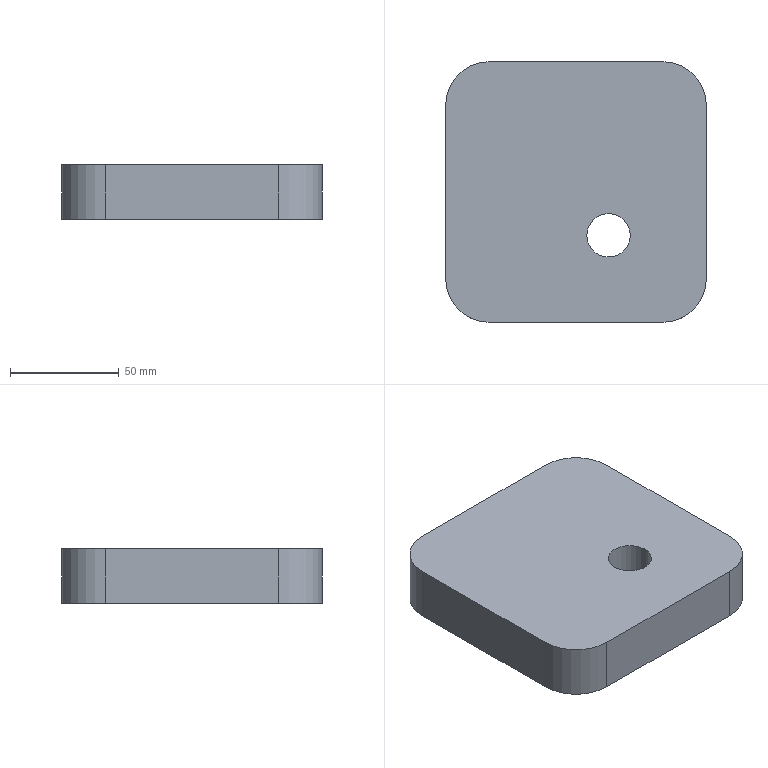Part | SolidWorks | features Extrusion 1, Fillet 1 | 1 solid | 12 faces | box 120 x 120 x 25 mm | volume 343562 mm3 | cylinder 6 | plane 6 | commonest cylinder face diameters 40 x4 20 x2
STEP:
#1=CARTESIAN_POINT('',(65.,40.,25.));
#2=VERTEX_POINT('',#1);
#3=CARTESIAN_POINT('',(85.,40.,25.));
#4=VERTEX_POINT('',#3);
#5=CARTESIAN_POINT('',(75.,40.,25.));
#6=DIRECTION('',(0.,0.,1.));
#7=DIRECTION('',(1.,0.,0.));
#8=AXIS2_PLACEMENT_3D('',#5,#6,#7);
#9=CIRCLE('',#8,10.);
#10=EDGE_CURVE('',#2,#4,#9,.T.);
#11=ORIENTED_EDGE('',*,*,#10,.T.);
#12=CARTESIAN_POINT('',(85.,40.,0.));
#13=VERTEX_POINT('',#12);
#14=CARTESIAN_POINT('',(85.,40.,25.));
#15=DIRECTION('',(0.,0.,-1.));
#16=VECTOR('',#15,1000.);
#17=LINE('',#14,#16);
#18=EDGE_CURVE('',#4,#13,#17,.T.);
#19=ORIENTED_EDGE('',*,*,#18,.T.);
#20=CARTESIAN_POINT('',(65.,40.,0.));
#21=VERTEX_POINT('',#20);
#22=CARTESIAN_POINT('',(75.,40.,0.));
#23=DIRECTION('',(0.,0.,1.));
#24=DIRECTION('',(1.,0.,0.));
#25=AXIS2_PLACEMENT_3D('',#22,#23,#24);
#26=CIRCLE('',#25,10.);
#27=EDGE_CURVE('',#21,#13,#26,.T.);
#28=ORIENTED_EDGE('',*,*,#27,.F.);
#29=CARTESIAN_POINT('',(65.,40.,25.));
#30=DIRECTION('',(0.,0.,-1.));
#31=VECTOR('',#30,1000.);
#32=LINE('',#29,#31);
#33=EDGE_CURVE('',#2,#21,#32,.T.);
#34=ORIENTED_EDGE('',*,*,#33,.F.);
#35=EDGE_LOOP('',(#11,#19,#28,#34));
#36=FACE_OUTER_BOUND('',#35,.T.);
#37=CARTESIAN_POINT('',(75.,40.,25.));
#38=DIRECTION('',(0.,0.,-1.));
#39=DIRECTION('',(-1.,0.,0.));
#40=AXIS2_PLACEMENT_3D('',#37,#38,#39);
#41=CYLINDRICAL_SURFACE('',#40,10.);
#42=ADVANCED_FACE('',(#36),#41,.F.);
#43=CARTESIAN_POINT('',(0.,100.,25.));
#44=VERTEX_POINT('',#43);
#45=CARTESIAN_POINT('',(0.,20.,25.));
#46=VERTEX_POINT('',#45);
#47=CARTESIAN_POINT('',(0.,0.,25.));
#48=DIRECTION('',(0.,-1.,0.));
#49=VECTOR('',#48,1000.);
#50=LINE('',#47,#49);
#51=EDGE_CURVE('',#44,#46,#50,.T.);
#52=ORIENTED_EDGE('',*,*,#51,.T.);
#53=CARTESIAN_POINT('',(20.,0.,25.));
#54=VERTEX_POINT('',#53);
#55=CARTESIAN_POINT('',(20.,20.,25.));
#56=DIRECTION('',(0.,0.,1.));
#57=DIRECTION('',(-1.,0.,0.));
#58=AXIS2_PLACEMENT_3D('',#55,#56,#57);
#59=CIRCLE('',#58,20.);
#60=EDGE_CURVE('',#46,#54,#59,.T.);
#61=ORIENTED_EDGE('',*,*,#60,.T.);
#62=CARTESIAN_POINT('',(100.,0.,25.));
#63=VERTEX_POINT('',#62);
#64=CARTESIAN_POINT('',(0.,0.,25.));
#65=DIRECTION('',(1.,0.,0.));
#66=VECTOR('',#65,1000.);
#67=LINE('',#64,#66);
#68=EDGE_CURVE('',#54,#63,#67,.T.);
#69=ORIENTED_EDGE('',*,*,#68,.T.);
#70=CARTESIAN_POINT('',(120.,20.,25.));
#71=VERTEX_POINT('',#70);
#72=CARTESIAN_POINT('',(100.,20.,25.));
#73=DIRECTION('',(0.,0.,1.));
#74=DIRECTION('',(-1.,0.,0.));
#75=AXIS2_PLACEMENT_3D('',#72,#73,#74);
#76=CIRCLE('',#75,20.);
#77=EDGE_CURVE('',#63,#71,#76,.T.);
#78=ORIENTED_EDGE('',*,*,#77,.T.);
#79=CARTESIAN_POINT('',(120.,100.,25.));
#80=VERTEX_POINT('',#79);
#81=CARTESIAN_POINT('',(120.,0.,25.));
#82=DIRECTION('',(0.,1.,0.));
#83=VECTOR('',#82,1000.);
#84=LINE('',#81,#83);
#85=EDGE_CURVE('',#71,#80,#84,.T.);
#86=ORIENTED_EDGE('',*,*,#85,.T.);
#87=CARTESIAN_POINT('',(100.,120.,25.));
#88=VERTEX_POINT('',#87);
#89=CARTESIAN_POINT('',(100.,100.,25.));
#90=DIRECTION('',(0.,0.,1.));
#91=DIRECTION('',(-1.,0.,0.));
#92=AXIS2_PLACEMENT_3D('',#89,#90,#91);
#93=CIRCLE('',#92,20.);
#94=EDGE_CURVE('',#80,#88,#93,.T.);
#95=ORIENTED_EDGE('',*,*,#94,.T.);
#96=CARTESIAN_POINT('',(20.,120.,25.));
#97=VERTEX_POINT('',#96);
#98=CARTESIAN_POINT('',(0.,120.,25.));
#99=DIRECTION('',(-1.,0.,0.));
#100=VECTOR('',#99,1000.);
#101=LINE('',#98,#100);
#102=EDGE_CURVE('',#88,#97,#101,.T.);
#103=ORIENTED_EDGE('',*,*,#102,.T.);
#104=CARTESIAN_POINT('',(20.,100.,25.));
#105=DIRECTION('',(0.,0.,1.));
#106=DIRECTION('',(-1.,0.,0.));
#107=AXIS2_PLACEMENT_3D('',#104,#105,#106);
#108=CIRCLE('',#107,20.);
#109=EDGE_CURVE('',#97,#44,#108,.T.);
#110=ORIENTED_EDGE('',*,*,#109,.T.);
#111=EDGE_LOOP('',(#52,#61,#69,#78,#86,#95,#103,#110));
#112=FACE_OUTER_BOUND('',#111,.T.);
#113=ORIENTED_EDGE('',*,*,#10,.F.);
#114=CARTESIAN_POINT('',(75.,40.,25.));
#115=DIRECTION('',(0.,0.,1.));
#116=DIRECTION('',(1.,0.,0.));
#117=AXIS2_PLACEMENT_3D('',#114,#115,#116);
#118=CIRCLE('',#117,10.);
#119=EDGE_CURVE('',#4,#2,#118,.T.);
#120=ORIENTED_EDGE('',*,*,#119,.F.);
#121=EDGE_LOOP('',(#113,#120));
#122=FACE_BOUND('',#121,.T.);
#123=CARTESIAN_POINT('',(0.,0.,25.));
#124=DIRECTION('',(0.,0.,-1.));
#125=DIRECTION('',(-1.,0.,0.));
#126=AXIS2_PLACEMENT_3D('',#123,#124,#125);
#127=PLANE('',#126);
#128=ADVANCED_FACE('',(#112,#122),#127,.F.);
#129=CARTESIAN_POINT('',(20.,0.,0.));
#130=VERTEX_POINT('',#129);
#131=CARTESIAN_POINT('',(100.,0.,0.));
#132=VERTEX_POINT('',#131);
#133=CARTESIAN_POINT('',(0.,0.,0.));
#134=DIRECTION('',(1.,0.,0.));
#135=VECTOR('',#134,1000.);
#136=LINE('',#133,#135);
#137=EDGE_CURVE('',#130,#132,#136,.T.);
#138=ORIENTED_EDGE('',*,*,#137,.F.);
#139=CARTESIAN_POINT('',(0.,20.,0.));
#140=VERTEX_POINT('',#139);
#141=CARTESIAN_POINT('',(20.,20.,0.));
#142=DIRECTION('',(0.,0.,-1.));
#143=DIRECTION('',(-1.,0.,0.));
#144=AXIS2_PLACEMENT_3D('',#141,#142,#143);
#145=CIRCLE('',#144,20.);
#146=EDGE_CURVE('',#130,#140,#145,.T.);
#147=ORIENTED_EDGE('',*,*,#146,.T.);
#148=CARTESIAN_POINT('',(0.,100.,0.));
#149=VERTEX_POINT('',#148);
#150=CARTESIAN_POINT('',(0.,0.,0.));
#151=DIRECTION('',(0.,-1.,0.));
#152=VECTOR('',#151,1000.);
#153=LINE('',#150,#152);
#154=EDGE_CURVE('',#149,#140,#153,.T.);
#155=ORIENTED_EDGE('',*,*,#154,.F.);
#156=CARTESIAN_POINT('',(20.,120.,0.));
#157=VERTEX_POINT('',#156);
#158=CARTESIAN_POINT('',(20.,100.,0.));
#159=DIRECTION('',(0.,0.,-1.));
#160=DIRECTION('',(-1.,0.,0.));
#161=AXIS2_PLACEMENT_3D('',#158,#159,#160);
#162=CIRCLE('',#161,20.);
#163=EDGE_CURVE('',#149,#157,#162,.T.);
#164=ORIENTED_EDGE('',*,*,#163,.T.);
#165=CARTESIAN_POINT('',(100.,120.,0.));
#166=VERTEX_POINT('',#165);
#167=CARTESIAN_POINT('',(0.,120.,0.));
#168=DIRECTION('',(-1.,0.,0.));
#169=VECTOR('',#168,1000.);
#170=LINE('',#167,#169);
#171=EDGE_CURVE('',#166,#157,#170,.T.);
#172=ORIENTED_EDGE('',*,*,#171,.F.);
#173=CARTESIAN_POINT('',(120.,100.,0.));
#174=VERTEX_POINT('',#173);
#175=CARTESIAN_POINT('',(100.,100.,0.));
#176=DIRECTION('',(0.,0.,-1.));
#177=DIRECTION('',(-1.,0.,0.));
#178=AXIS2_PLACEMENT_3D('',#175,#176,#177);
#179=CIRCLE('',#178,20.);
#180=EDGE_CURVE('',#166,#174,#179,.T.);
#181=ORIENTED_EDGE('',*,*,#180,.T.);
#182=CARTESIAN_POINT('',(120.,20.,0.));
#183=VERTEX_POINT('',#182);
#184=CARTESIAN_POINT('',(120.,0.,0.));
#185=DIRECTION('',(0.,1.,0.));
#186=VECTOR('',#185,1000.);
#187=LINE('',#184,#186);
#188=EDGE_CURVE('',#183,#174,#187,.T.);
#189=ORIENTED_EDGE('',*,*,#188,.F.);
#190=CARTESIAN_POINT('',(100.,20.,0.));
#191=DIRECTION('',(0.,0.,-1.));
#192=DIRECTION('',(-1.,0.,0.));
#193=AXIS2_PLACEMENT_3D('',#190,#191,#192);
#194=CIRCLE('',#193,20.);
#195=EDGE_CURVE('',#183,#132,#194,.T.);
#196=ORIENTED_EDGE('',*,*,#195,.T.);
#197=EDGE_LOOP('',(#138,#147,#155,#164,#172,#181,#189,#196));
#198=FACE_OUTER_BOUND('',#197,.T.);
#199=ORIENTED_EDGE('',*,*,#27,.T.);
#200=CARTESIAN_POINT('',(75.,40.,0.));
#201=DIRECTION('',(0.,0.,1.));
#202=DIRECTION('',(1.,0.,0.));
#203=AXIS2_PLACEMENT_3D('',#200,#201,#202);
#204=CIRCLE('',#203,10.);
#205=EDGE_CURVE('',#13,#21,#204,.T.);
#206=ORIENTED_EDGE('',*,*,#205,.T.);
#207=EDGE_LOOP('',(#199,#206));
#208=FACE_BOUND('',#207,.T.);
#209=CARTESIAN_POINT('',(0.,0.,0.));
#210=DIRECTION('',(0.,0.,-1.));
#211=DIRECTION('',(-1.,0.,0.));
#212=AXIS2_PLACEMENT_3D('',#209,#210,#211);
#213=PLANE('',#212);
#214=ADVANCED_FACE('',(#198,#208),#213,.T.);
#215=ORIENTED_EDGE('',*,*,#154,.T.);
#216=CARTESIAN_POINT('',(0.,20.,25.));
#217=DIRECTION('',(0.,0.,1.));
#218=VECTOR('',#217,1000.);
#219=LINE('',#216,#218);
#220=EDGE_CURVE('',#140,#46,#219,.T.);
#221=ORIENTED_EDGE('',*,*,#220,.T.);
#222=ORIENTED_EDGE('',*,*,#51,.F.);
#223=CARTESIAN_POINT('',(0.,100.,25.));
#224=DIRECTION('',(0.,0.,-1.));
#225=VECTOR('',#224,1000.);
#226=LINE('',#223,#225);
#227=EDGE_CURVE('',#44,#149,#226,.T.);
#228=ORIENTED_EDGE('',*,*,#227,.T.);
#229=EDGE_LOOP('',(#215,#221,#222,#228));
#230=FACE_OUTER_BOUND('',#229,.T.);
#231=CARTESIAN_POINT('',(0.,0.,25.));
#232=DIRECTION('',(1.,0.,0.));
#233=DIRECTION('',(0.,0.,-1.));
#234=AXIS2_PLACEMENT_3D('',#231,#232,#233);
#235=PLANE('',#234);
#236=ADVANCED_FACE('',(#230),#235,.F.);
#237=ORIENTED_EDGE('',*,*,#68,.F.);
#238=CARTESIAN_POINT('',(20.,0.,25.));
#239=DIRECTION('',(0.,0.,-1.));
#240=VECTOR('',#239,1000.);
#241=LINE('',#238,#240);
#242=EDGE_CURVE('',#54,#130,#241,.T.);
#243=ORIENTED_EDGE('',*,*,#242,.T.);
#244=ORIENTED_EDGE('',*,*,#137,.T.);
#245=CARTESIAN_POINT('',(100.,0.,25.));
#246=DIRECTION('',(0.,0.,1.));
#247=VECTOR('',#246,1000.);
#248=LINE('',#245,#247);
#249=EDGE_CURVE('',#132,#63,#248,.T.);
#250=ORIENTED_EDGE('',*,*,#249,.T.);
#251=EDGE_LOOP('',(#237,#243,#244,#250));
#252=FACE_OUTER_BOUND('',#251,.T.);
#253=CARTESIAN_POINT('',(0.,0.,25.));
#254=DIRECTION('',(0.,1.,0.));
#255=DIRECTION('',(0.,0.,1.));
#256=AXIS2_PLACEMENT_3D('',#253,#254,#255);
#257=PLANE('',#256);
#258=ADVANCED_FACE('',(#252),#257,.F.);
#259=ORIENTED_EDGE('',*,*,#85,.F.);
#260=CARTESIAN_POINT('',(120.,20.,25.));
#261=DIRECTION('',(0.,0.,-1.));
#262=VECTOR('',#261,1000.);
#263=LINE('',#260,#262);
#264=EDGE_CURVE('',#71,#183,#263,.T.);
#265=ORIENTED_EDGE('',*,*,#264,.T.);
#266=ORIENTED_EDGE('',*,*,#188,.T.);
#267=CARTESIAN_POINT('',(120.,100.,25.));
#268=DIRECTION('',(0.,0.,1.));
#269=VECTOR('',#268,1000.);
#270=LINE('',#267,#269);
#271=EDGE_CURVE('',#174,#80,#270,.T.);
#272=ORIENTED_EDGE('',*,*,#271,.T.);
#273=EDGE_LOOP('',(#259,#265,#266,#272));
#274=FACE_OUTER_BOUND('',#273,.T.);
#275=CARTESIAN_POINT('',(120.,0.,25.));
#276=DIRECTION('',(-1.,0.,0.));
#277=DIRECTION('',(0.,0.,1.));
#278=AXIS2_PLACEMENT_3D('',#275,#276,#277);
#279=PLANE('',#278);
#280=ADVANCED_FACE('',(#274),#279,.F.);
#281=ORIENTED_EDGE('',*,*,#102,.F.);
#282=CARTESIAN_POINT('',(100.,120.,25.));
#283=DIRECTION('',(0.,0.,-1.));
#284=VECTOR('',#283,1000.);
#285=LINE('',#282,#284);
#286=EDGE_CURVE('',#88,#166,#285,.T.);
#287=ORIENTED_EDGE('',*,*,#286,.T.);
#288=ORIENTED_EDGE('',*,*,#171,.T.);
#289=CARTESIAN_POINT('',(20.,120.,25.));
#290=DIRECTION('',(0.,0.,1.));
#291=VECTOR('',#290,1000.);
#292=LINE('',#289,#291);
#293=EDGE_CURVE('',#157,#97,#292,.T.);
#294=ORIENTED_EDGE('',*,*,#293,.T.);
#295=EDGE_LOOP('',(#281,#287,#288,#294));
#296=FACE_OUTER_BOUND('',#295,.T.);
#297=CARTESIAN_POINT('',(0.,120.,25.));
#298=DIRECTION('',(0.,-1.,0.));
#299=DIRECTION('',(0.,0.,-1.));
#300=AXIS2_PLACEMENT_3D('',#297,#298,#299);
#301=PLANE('',#300);
#302=ADVANCED_FACE('',(#296),#301,.F.);
#303=ORIENTED_EDGE('',*,*,#18,.F.);
#304=ORIENTED_EDGE('',*,*,#119,.T.);
#305=ORIENTED_EDGE('',*,*,#33,.T.);
#306=ORIENTED_EDGE('',*,*,#205,.F.);
#307=EDGE_LOOP('',(#303,#304,#305,#306));
#308=FACE_OUTER_BOUND('',#307,.T.);
#309=CARTESIAN_POINT('',(75.,40.,25.));
#310=DIRECTION('',(0.,0.,-1.));
#311=DIRECTION('',(-1.,0.,0.));
#312=AXIS2_PLACEMENT_3D('',#309,#310,#311);
#313=CYLINDRICAL_SURFACE('',#312,10.);
#314=ADVANCED_FACE('',(#308),#313,.F.);
#315=ORIENTED_EDGE('',*,*,#60,.F.);
#316=ORIENTED_EDGE('',*,*,#220,.F.);
#317=ORIENTED_EDGE('',*,*,#146,.F.);
#318=ORIENTED_EDGE('',*,*,#242,.F.);
#319=EDGE_LOOP('',(#315,#316,#317,#318));
#320=FACE_OUTER_BOUND('',#319,.T.);
#321=CARTESIAN_POINT('',(20.,20.,25.));
#322=DIRECTION('',(0.,0.,-1.));
#323=DIRECTION('',(-1.,0.,0.));
#324=AXIS2_PLACEMENT_3D('',#321,#322,#323);
#325=CYLINDRICAL_SURFACE('',#324,20.);
#326=ADVANCED_FACE('',(#320),#325,.T.);
#327=ORIENTED_EDGE('',*,*,#77,.F.);
#328=ORIENTED_EDGE('',*,*,#249,.F.);
#329=ORIENTED_EDGE('',*,*,#195,.F.);
#330=ORIENTED_EDGE('',*,*,#264,.F.);
#331=EDGE_LOOP('',(#327,#328,#329,#330));
#332=FACE_OUTER_BOUND('',#331,.T.);
#333=CARTESIAN_POINT('',(100.,20.,25.));
#334=DIRECTION('',(0.,0.,-1.));
#335=DIRECTION('',(-1.,0.,0.));
#336=AXIS2_PLACEMENT_3D('',#333,#334,#335);
#337=CYLINDRICAL_SURFACE('',#336,20.);
#338=ADVANCED_FACE('',(#332),#337,.T.);
#339=ORIENTED_EDGE('',*,*,#94,.F.);
#340=ORIENTED_EDGE('',*,*,#271,.F.);
#341=ORIENTED_EDGE('',*,*,#180,.F.);
#342=ORIENTED_EDGE('',*,*,#286,.F.);
#343=EDGE_LOOP('',(#339,#340,#341,#342));
#344=FACE_OUTER_BOUND('',#343,.T.);
#345=CARTESIAN_POINT('',(100.,100.,25.));
#346=DIRECTION('',(0.,0.,-1.));
#347=DIRECTION('',(-1.,0.,0.));
#348=AXIS2_PLACEMENT_3D('',#345,#346,#347);
#349=CYLINDRICAL_SURFACE('',#348,20.);
#350=ADVANCED_FACE('',(#344),#349,.T.);
#351=ORIENTED_EDGE('',*,*,#109,.F.);
#352=ORIENTED_EDGE('',*,*,#293,.F.);
#353=ORIENTED_EDGE('',*,*,#163,.F.);
#354=ORIENTED_EDGE('',*,*,#227,.F.);
#355=EDGE_LOOP('',(#351,#352,#353,#354));
#356=FACE_OUTER_BOUND('',#355,.T.);
#357=CARTESIAN_POINT('',(20.,100.,25.));
#358=DIRECTION('',(0.,0.,-1.));
#359=DIRECTION('',(-1.,0.,0.));
#360=AXIS2_PLACEMENT_3D('',#357,#358,#359);
#361=CYLINDRICAL_SURFACE('',#360,20.);
#362=ADVANCED_FACE('',(#356),#361,.T.);
#363=CLOSED_SHELL('',(#42,#128,#214,#236,#258,#280,#302,#314,#326,#338,#350,#362));
#364=MANIFOLD_SOLID_BREP('',#363);
#365=CARTESIAN_POINT('',(0.,0.,0.));
#366=DIRECTION('',(0.,0.,1.));
#367=DIRECTION('',(1.,0.,0.));
#368=AXIS2_PLACEMENT_3D('',#365,#366,#367);
#369=(LENGTH_UNIT()NAMED_UNIT(*)SI_UNIT(.MILLI.,.METRE.));
#370=UNCERTAINTY_MEASURE_WITH_UNIT(LENGTH_MEASURE(0.00001),#369,'','');
#371=(NAMED_UNIT(*)PLANE_ANGLE_UNIT()SI_UNIT($,.RADIAN.));
#372=(NAMED_UNIT(*)SI_UNIT($,.STERADIAN.)SOLID_ANGLE_UNIT());
#373=(GEOMETRIC_REPRESENTATION_CONTEXT(3)GLOBAL_UNCERTAINTY_ASSIGNED_CONTEXT((#370))GLOBAL_UNIT_ASSIGNED_CONTEXT((#369,#371,#372))REPRESENTATION_CONTEXT('',''));
#374=ADVANCED_BREP_SHAPE_REPRESENTATION('',(#364,#368),#373);